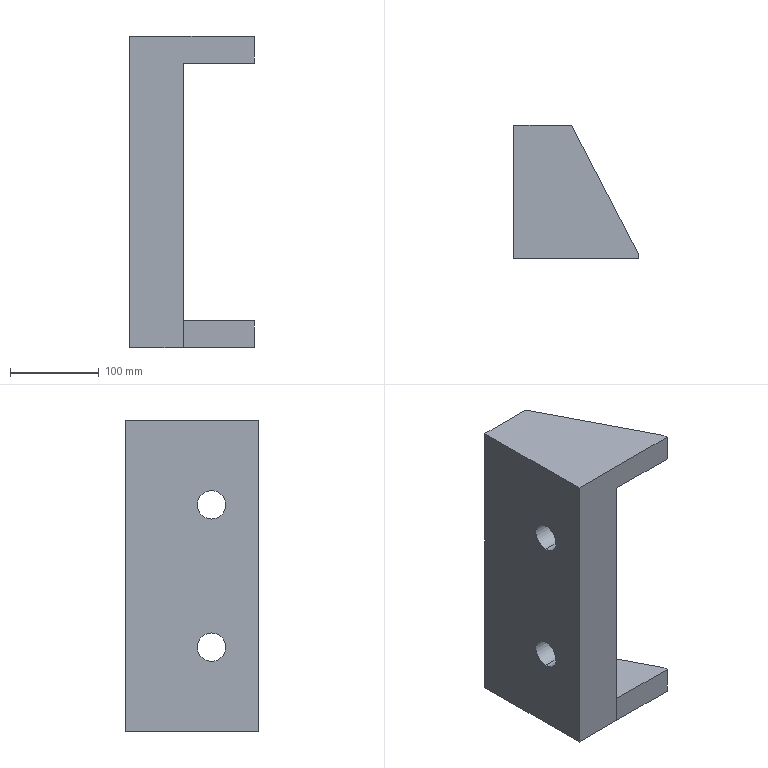Part | STEP file | PN_0005 Linear bearing seat | 2 solids | 20 faces | box 140 x 150 x 350 mm | volume 3447240 mm3 | plane 16 | cylinder 4 | commonest cylinder face diameters 32 x4
STEP:
#1=CARTESIAN_POINT('',(0.,0.,0.));
#2=DIRECTION('',(0.,0.,1.));
#3=DIRECTION('',(1.,0.,0.));
#4=AXIS2_PLACEMENT_3D('',#1,#2,#3);
#5=CARTESIAN_POINT('',(110.,0.,-175.));
#6=VERTEX_POINT('',#5);
#7=CARTESIAN_POINT('',(30.,0.,-175.));
#8=VERTEX_POINT('',#7);
#9=CARTESIAN_POINT('',(30.,0.,-175.));
#10=DIRECTION('',(-1.,0.,0.));
#11=VECTOR('',#10,1.);
#12=LINE('',#9,#11);
#13=CARTESIAN_POINT('',(30.,0.,-145.));
#14=DIRECTION('',(0.,-1.,0.));
#15=DIRECTION('',(1.,0.,0.));
#16=AXIS2_PLACEMENT_3D('',#13,#14,#15);
#17=PLANE('',#16);
#18=CARTESIAN_POINT('',(0.,-30.));
#19=DIRECTION('',(-1.,0.));
#20=VECTOR('',#19,1.);
#21=LINE('',#18,#20);
#22=(GEOMETRIC_REPRESENTATION_CONTEXT(2)PARAMETRIC_REPRESENTATION_CONTEXT()REPRESENTATION_CONTEXT('',''));
#23=DEFINITIONAL_REPRESENTATION('',(#21),#22);
#24=PCURVE('',#17,#23);
#25=CARTESIAN_POINT('',(110.,0.,-175.));
#26=DIRECTION('',(0.,0.,-1.));
#27=DIRECTION('',(-1.,0.,0.));
#28=AXIS2_PLACEMENT_3D('',#25,#26,#27);
#29=PLANE('',#28);
#30=CARTESIAN_POINT('',(80.,0.));
#31=DIRECTION('',(1.,0.));
#32=VECTOR('',#31,1.);
#33=LINE('',#30,#32);
#34=(GEOMETRIC_REPRESENTATION_CONTEXT(2)PARAMETRIC_REPRESENTATION_CONTEXT()REPRESENTATION_CONTEXT('',''));
#35=DEFINITIONAL_REPRESENTATION('',(#33),#34);
#36=PCURVE('',#29,#35);
#37=SURFACE_CURVE('',#12,(#24,#36),.PCURVE_S1.);
#38=EDGE_CURVE('',#6,#8,#37,.T.);
#39=ORIENTED_EDGE('',*,*,#38,.F.);
#40=CARTESIAN_POINT('',(110.,0.,-145.));
#41=VERTEX_POINT('',#40);
#42=CARTESIAN_POINT('',(110.,0.,-145.));
#43=DIRECTION('',(0.,0.,-1.));
#44=VECTOR('',#43,1.);
#45=LINE('',#42,#44);
#46=CARTESIAN_POINT('',(80.,0.));
#47=DIRECTION('',(0.,-1.));
#48=VECTOR('',#47,1.);
#49=LINE('',#46,#48);
#50=(GEOMETRIC_REPRESENTATION_CONTEXT(2)PARAMETRIC_REPRESENTATION_CONTEXT()REPRESENTATION_CONTEXT('',''));
#51=DEFINITIONAL_REPRESENTATION('',(#49),#50);
#52=PCURVE('',#17,#51);
#53=CARTESIAN_POINT('',(110.,5.,-145.));
#54=DIRECTION('',(1.,0.,0.));
#55=DIRECTION('',(0.,0.,-1.));
#56=AXIS2_PLACEMENT_3D('',#53,#54,#55);
#57=PLANE('',#56);
#58=CARTESIAN_POINT('',(0.,-5.));
#59=DIRECTION('',(1.,0.));
#60=VECTOR('',#59,1.);
#61=LINE('',#58,#60);
#62=(GEOMETRIC_REPRESENTATION_CONTEXT(2)PARAMETRIC_REPRESENTATION_CONTEXT()REPRESENTATION_CONTEXT('',''));
#63=DEFINITIONAL_REPRESENTATION('',(#61),#62);
#64=PCURVE('',#57,#63);
#65=SURFACE_CURVE('',#45,(#52,#64),.PCURVE_S1.);
#66=EDGE_CURVE('',#41,#6,#65,.T.);
#67=ORIENTED_EDGE('',*,*,#66,.F.);
#68=CARTESIAN_POINT('',(30.,0.,-145.));
#69=VERTEX_POINT('',#68);
#70=CARTESIAN_POINT('',(30.,0.,-145.));
#71=DIRECTION('',(-1.,0.,0.));
#72=VECTOR('',#71,1.);
#73=LINE('',#70,#72);
#74=CARTESIAN_POINT('',(0.,0.));
#75=DIRECTION('',(-1.,0.));
#76=VECTOR('',#75,1.);
#77=LINE('',#74,#76);
#78=(GEOMETRIC_REPRESENTATION_CONTEXT(2)PARAMETRIC_REPRESENTATION_CONTEXT()REPRESENTATION_CONTEXT('',''));
#79=DEFINITIONAL_REPRESENTATION('',(#77),#78);
#80=PCURVE('',#17,#79);
#81=CARTESIAN_POINT('',(110.,0.,-145.));
#82=DIRECTION('',(0.,0.,-1.));
#83=DIRECTION('',(-1.,0.,0.));
#84=AXIS2_PLACEMENT_3D('',#81,#82,#83);
#85=PLANE('',#84);
#86=CARTESIAN_POINT('',(80.,0.));
#87=DIRECTION('',(1.,0.));
#88=VECTOR('',#87,1.);
#89=LINE('',#86,#88);
#90=(GEOMETRIC_REPRESENTATION_CONTEXT(2)PARAMETRIC_REPRESENTATION_CONTEXT()REPRESENTATION_CONTEXT('',''));
#91=DEFINITIONAL_REPRESENTATION('',(#89),#90);
#92=PCURVE('',#85,#91);
#93=SURFACE_CURVE('',#73,(#80,#92),.PCURVE_S1.);
#94=EDGE_CURVE('',#41,#69,#93,.T.);
#95=ORIENTED_EDGE('',*,*,#94,.T.);
#96=CARTESIAN_POINT('',(30.,0.,-145.));
#97=DIRECTION('',(0.,0.,-1.));
#98=VECTOR('',#97,1.);
#99=LINE('',#96,#98);
#100=CARTESIAN_POINT('',(0.,0.));
#101=DIRECTION('',(0.,-1.));
#102=VECTOR('',#101,1.);
#103=LINE('',#100,#102);
#104=(GEOMETRIC_REPRESENTATION_CONTEXT(2)PARAMETRIC_REPRESENTATION_CONTEXT()REPRESENTATION_CONTEXT('',''));
#105=DEFINITIONAL_REPRESENTATION('',(#103),#104);
#106=PCURVE('',#17,#105);
#107=CARTESIAN_POINT('',(30.,150.,-145.));
#108=DIRECTION('',(-1.,0.,0.));
#109=DIRECTION('',(0.,0.,1.));
#110=AXIS2_PLACEMENT_3D('',#107,#108,#109);
#111=PLANE('',#110);
#112=CARTESIAN_POINT('',(0.,-150.));
#113=DIRECTION('',(-1.,0.));
#114=VECTOR('',#113,1.);
#115=LINE('',#112,#114);
#116=(GEOMETRIC_REPRESENTATION_CONTEXT(2)PARAMETRIC_REPRESENTATION_CONTEXT()REPRESENTATION_CONTEXT('',''));
#117=DEFINITIONAL_REPRESENTATION('',(#115),#116);
#118=PCURVE('',#111,#117);
#119=SURFACE_CURVE('',#99,(#106,#118),.PCURVE_S1.);
#120=EDGE_CURVE('',#69,#8,#119,.T.);
#121=ORIENTED_EDGE('',*,*,#120,.T.);
#122=EDGE_LOOP('',(#39,#67,#95,#121));
#123=FACE_BOUND('',#122,.T.);
#124=ADVANCED_FACE('',(#123),#17,.T.);
#125=CARTESIAN_POINT('',(110.,5.,-175.));
#126=VERTEX_POINT('',#125);
#127=CARTESIAN_POINT('',(110.,5.,-175.));
#128=DIRECTION('',(0.,-1.,0.));
#129=VECTOR('',#128,1.);
#130=LINE('',#127,#129);
#131=CARTESIAN_POINT('',(30.,0.));
#132=DIRECTION('',(0.,-1.));
#133=VECTOR('',#132,1.);
#134=LINE('',#131,#133);
#135=(GEOMETRIC_REPRESENTATION_CONTEXT(2)PARAMETRIC_REPRESENTATION_CONTEXT()REPRESENTATION_CONTEXT('',''));
#136=DEFINITIONAL_REPRESENTATION('',(#134),#135);
#137=PCURVE('',#57,#136);
#138=CARTESIAN_POINT('',(0.,5.));
#139=DIRECTION('',(0.,-1.));
#140=VECTOR('',#139,1.);
#141=LINE('',#138,#140);
#142=(GEOMETRIC_REPRESENTATION_CONTEXT(2)PARAMETRIC_REPRESENTATION_CONTEXT()REPRESENTATION_CONTEXT('',''));
#143=DEFINITIONAL_REPRESENTATION('',(#141),#142);
#144=PCURVE('',#29,#143);
#145=SURFACE_CURVE('',#130,(#137,#144),.PCURVE_S1.);
#146=EDGE_CURVE('',#126,#6,#145,.T.);
#147=ORIENTED_EDGE('',*,*,#146,.F.);
#148=CARTESIAN_POINT('',(110.,5.,-145.));
#149=VERTEX_POINT('',#148);
#150=CARTESIAN_POINT('',(110.,5.,-145.));
#151=DIRECTION('',(0.,0.,-1.));
#152=VECTOR('',#151,1.);
#153=LINE('',#150,#152);
#154=CARTESIAN_POINT('',(0.,0.));
#155=DIRECTION('',(1.,0.));
#156=VECTOR('',#155,1.);
#157=LINE('',#154,#156);
#158=(GEOMETRIC_REPRESENTATION_CONTEXT(2)PARAMETRIC_REPRESENTATION_CONTEXT()REPRESENTATION_CONTEXT('',''));
#159=DEFINITIONAL_REPRESENTATION('',(#157),#158);
#160=PCURVE('',#57,#159);
#161=CARTESIAN_POINT('',(110.,5.,-145.));
#162=DIRECTION('',(0.8882,0.4594,0.));
#163=DIRECTION('',(-0.4594,0.8882,0.));
#164=AXIS2_PLACEMENT_3D('',#161,#162,#163);
#165=PLANE('',#164);
#166=CARTESIAN_POINT('',(0.,0.));
#167=DIRECTION('',(0.,-1.));
#168=VECTOR('',#167,1.);
#169=LINE('',#166,#168);
#170=(GEOMETRIC_REPRESENTATION_CONTEXT(2)PARAMETRIC_REPRESENTATION_CONTEXT()REPRESENTATION_CONTEXT('',''));
#171=DEFINITIONAL_REPRESENTATION('',(#169),#170);
#172=PCURVE('',#165,#171);
#173=SURFACE_CURVE('',#153,(#160,#172),.PCURVE_S1.);
#174=EDGE_CURVE('',#149,#126,#173,.T.);
#175=ORIENTED_EDGE('',*,*,#174,.F.);
#176=CARTESIAN_POINT('',(110.,5.,-145.));
#177=DIRECTION('',(0.,-1.,0.));
#178=VECTOR('',#177,1.);
#179=LINE('',#176,#178);
#180=CARTESIAN_POINT('',(0.,0.));
#181=DIRECTION('',(0.,-1.));
#182=VECTOR('',#181,1.);
#183=LINE('',#180,#182);
#184=(GEOMETRIC_REPRESENTATION_CONTEXT(2)PARAMETRIC_REPRESENTATION_CONTEXT()REPRESENTATION_CONTEXT('',''));
#185=DEFINITIONAL_REPRESENTATION('',(#183),#184);
#186=PCURVE('',#57,#185);
#187=CARTESIAN_POINT('',(0.,5.));
#188=DIRECTION('',(0.,-1.));
#189=VECTOR('',#188,1.);
#190=LINE('',#187,#189);
#191=(GEOMETRIC_REPRESENTATION_CONTEXT(2)PARAMETRIC_REPRESENTATION_CONTEXT()REPRESENTATION_CONTEXT('',''));
#192=DEFINITIONAL_REPRESENTATION('',(#190),#191);
#193=PCURVE('',#85,#192);
#194=SURFACE_CURVE('',#179,(#186,#193),.PCURVE_S1.);
#195=EDGE_CURVE('',#149,#41,#194,.T.);
#196=ORIENTED_EDGE('',*,*,#195,.T.);
#197=ORIENTED_EDGE('',*,*,#66,.T.);
#198=EDGE_LOOP('',(#147,#175,#196,#197));
#199=FACE_BOUND('',#198,.T.);
#200=ADVANCED_FACE('',(#199),#57,.T.);
#201=CARTESIAN_POINT('',(35.,150.,-175.));
#202=VERTEX_POINT('',#201);
#203=CARTESIAN_POINT('',(110.,5.,-175.));
#204=DIRECTION('',(0.4594,-0.8882,0.));
#205=VECTOR('',#204,1.);
#206=LINE('',#203,#205);
#207=CARTESIAN_POINT('',(0.,-30.));
#208=DIRECTION('',(-1.,0.));
#209=VECTOR('',#208,1.);
#210=LINE('',#207,#209);
#211=(GEOMETRIC_REPRESENTATION_CONTEXT(2)PARAMETRIC_REPRESENTATION_CONTEXT()REPRESENTATION_CONTEXT('',''));
#212=DEFINITIONAL_REPRESENTATION('',(#210),#211);
#213=PCURVE('',#165,#212);
#214=CARTESIAN_POINT('',(0.,5.));
#215=DIRECTION('',(-0.4594,-0.8882));
#216=VECTOR('',#215,1.);
#217=LINE('',#214,#216);
#218=(GEOMETRIC_REPRESENTATION_CONTEXT(2)PARAMETRIC_REPRESENTATION_CONTEXT()REPRESENTATION_CONTEXT('',''));
#219=DEFINITIONAL_REPRESENTATION('',(#217),#218);
#220=PCURVE('',#29,#219);
#221=SURFACE_CURVE('',#206,(#213,#220),.PCURVE_S1.);
#222=EDGE_CURVE('',#202,#126,#221,.T.);
#223=ORIENTED_EDGE('',*,*,#222,.F.);
#224=CARTESIAN_POINT('',(35.,150.,-145.));
#225=VERTEX_POINT('',#224);
#226=CARTESIAN_POINT('',(35.,150.,-145.));
#227=DIRECTION('',(0.,0.,-1.));
#228=VECTOR('',#227,1.);
#229=LINE('',#226,#228);
#230=CARTESIAN_POINT('',(163.248,0.));
#231=DIRECTION('',(0.,-1.));
#232=VECTOR('',#231,1.);
#233=LINE('',#230,#232);
#234=(GEOMETRIC_REPRESENTATION_CONTEXT(2)PARAMETRIC_REPRESENTATION_CONTEXT()REPRESENTATION_CONTEXT('',''));
#235=DEFINITIONAL_REPRESENTATION('',(#233),#234);
#236=PCURVE('',#165,#235);
#237=CARTESIAN_POINT('',(35.,150.,-145.));
#238=DIRECTION('',(0.,1.,0.));
#239=DIRECTION('',(-1.,0.,0.));
#240=AXIS2_PLACEMENT_3D('',#237,#238,#239);
#241=PLANE('',#240);
#242=CARTESIAN_POINT('',(0.,0.));
#243=DIRECTION('',(0.,-1.));
#244=VECTOR('',#243,1.);
#245=LINE('',#242,#244);
#246=(GEOMETRIC_REPRESENTATION_CONTEXT(2)PARAMETRIC_REPRESENTATION_CONTEXT()REPRESENTATION_CONTEXT('',''));
#247=DEFINITIONAL_REPRESENTATION('',(#245),#246);
#248=PCURVE('',#241,#247);
#249=SURFACE_CURVE('',#229,(#236,#248),.PCURVE_S1.);
#250=EDGE_CURVE('',#225,#202,#249,.T.);
#251=ORIENTED_EDGE('',*,*,#250,.F.);
#252=CARTESIAN_POINT('',(110.,5.,-145.));
#253=DIRECTION('',(0.4594,-0.8882,0.));
#254=VECTOR('',#253,1.);
#255=LINE('',#252,#254);
#256=CARTESIAN_POINT('',(0.,0.));
#257=DIRECTION('',(-1.,0.));
#258=VECTOR('',#257,1.);
#259=LINE('',#256,#258);
#260=(GEOMETRIC_REPRESENTATION_CONTEXT(2)PARAMETRIC_REPRESENTATION_CONTEXT()REPRESENTATION_CONTEXT('',''));
#261=DEFINITIONAL_REPRESENTATION('',(#259),#260);
#262=PCURVE('',#165,#261);
#263=CARTESIAN_POINT('',(0.,5.));
#264=DIRECTION('',(-0.4594,-0.8882));
#265=VECTOR('',#264,1.);
#266=LINE('',#263,#265);
#267=(GEOMETRIC_REPRESENTATION_CONTEXT(2)PARAMETRIC_REPRESENTATION_CONTEXT()REPRESENTATION_CONTEXT('',''));
#268=DEFINITIONAL_REPRESENTATION('',(#266),#267);
#269=PCURVE('',#85,#268);
#270=SURFACE_CURVE('',#255,(#262,#269),.PCURVE_S1.);
#271=EDGE_CURVE('',#225,#149,#270,.T.);
#272=ORIENTED_EDGE('',*,*,#271,.T.);
#273=ORIENTED_EDGE('',*,*,#174,.T.);
#274=EDGE_LOOP('',(#223,#251,#272,#273));
#275=FACE_BOUND('',#274,.T.);
#276=ADVANCED_FACE('',(#275),#165,.T.);
#277=CARTESIAN_POINT('',(30.,150.,-175.));
#278=VERTEX_POINT('',#277);
#279=CARTESIAN_POINT('',(35.,150.,-175.));
#280=DIRECTION('',(1.,0.,0.));
#281=VECTOR('',#280,1.);
#282=LINE('',#279,#281);
#283=CARTESIAN_POINT('',(0.,-30.));
#284=DIRECTION('',(-1.,0.));
#285=VECTOR('',#284,1.);
#286=LINE('',#283,#285);
#287=(GEOMETRIC_REPRESENTATION_CONTEXT(2)PARAMETRIC_REPRESENTATION_CONTEXT()REPRESENTATION_CONTEXT('',''));
#288=DEFINITIONAL_REPRESENTATION('',(#286),#287);
#289=PCURVE('',#241,#288);
#290=CARTESIAN_POINT('',(75.,150.));
#291=DIRECTION('',(-1.,0.));
#292=VECTOR('',#291,1.);
#293=LINE('',#290,#292);
#294=(GEOMETRIC_REPRESENTATION_CONTEXT(2)PARAMETRIC_REPRESENTATION_CONTEXT()REPRESENTATION_CONTEXT('',''));
#295=DEFINITIONAL_REPRESENTATION('',(#293),#294);
#296=PCURVE('',#29,#295);
#297=SURFACE_CURVE('',#282,(#289,#296),.PCURVE_S1.);
#298=EDGE_CURVE('',#278,#202,#297,.T.);
#299=ORIENTED_EDGE('',*,*,#298,.F.);
#300=CARTESIAN_POINT('',(30.,150.,-145.));
#301=VERTEX_POINT('',#300);
#302=CARTESIAN_POINT('',(30.,150.,-145.));
#303=DIRECTION('',(0.,0.,-1.));
#304=VECTOR('',#303,1.);
#305=LINE('',#302,#304);
#306=CARTESIAN_POINT('',(5.,0.));
#307=DIRECTION('',(0.,-1.));
#308=VECTOR('',#307,1.);
#309=LINE('',#306,#308);
#310=(GEOMETRIC_REPRESENTATION_CONTEXT(2)PARAMETRIC_REPRESENTATION_CONTEXT()REPRESENTATION_CONTEXT('',''));
#311=DEFINITIONAL_REPRESENTATION('',(#309),#310);
#312=PCURVE('',#241,#311);
#313=CARTESIAN_POINT('',(0.,0.));
#314=DIRECTION('',(-1.,0.));
#315=VECTOR('',#314,1.);
#316=LINE('',#313,#315);
#317=(GEOMETRIC_REPRESENTATION_CONTEXT(2)PARAMETRIC_REPRESENTATION_CONTEXT()REPRESENTATION_CONTEXT('',''));
#318=DEFINITIONAL_REPRESENTATION('',(#316),#317);
#319=PCURVE('',#111,#318);
#320=SURFACE_CURVE('',#305,(#312,#319),.PCURVE_S1.);
#321=EDGE_CURVE('',#301,#278,#320,.T.);
#322=ORIENTED_EDGE('',*,*,#321,.F.);
#323=CARTESIAN_POINT('',(35.,150.,-145.));
#324=DIRECTION('',(1.,0.,0.));
#325=VECTOR('',#324,1.);
#326=LINE('',#323,#325);
#327=CARTESIAN_POINT('',(0.,0.));
#328=DIRECTION('',(-1.,0.));
#329=VECTOR('',#328,1.);
#330=LINE('',#327,#329);
#331=(GEOMETRIC_REPRESENTATION_CONTEXT(2)PARAMETRIC_REPRESENTATION_CONTEXT()REPRESENTATION_CONTEXT('',''));
#332=DEFINITIONAL_REPRESENTATION('',(#330),#331);
#333=PCURVE('',#241,#332);
#334=CARTESIAN_POINT('',(75.,150.));
#335=DIRECTION('',(-1.,0.));
#336=VECTOR('',#335,1.);
#337=LINE('',#334,#336);
#338=(GEOMETRIC_REPRESENTATION_CONTEXT(2)PARAMETRIC_REPRESENTATION_CONTEXT()REPRESENTATION_CONTEXT('',''));
#339=DEFINITIONAL_REPRESENTATION('',(#337),#338);
#340=PCURVE('',#85,#339);
#341=SURFACE_CURVE('',#326,(#333,#340),.PCURVE_S1.);
#342=EDGE_CURVE('',#301,#225,#341,.T.);
#343=ORIENTED_EDGE('',*,*,#342,.T.);
#344=ORIENTED_EDGE('',*,*,#250,.T.);
#345=EDGE_LOOP('',(#299,#322,#343,#344));
#346=FACE_BOUND('',#345,.T.);
#347=ADVANCED_FACE('',(#346),#241,.T.);
#348=CARTESIAN_POINT('',(30.,150.,-175.));
#349=DIRECTION('',(0.,1.,0.));
#350=VECTOR('',#349,1.);
#351=LINE('',#348,#350);
#352=CARTESIAN_POINT('',(-30.,0.));
#353=DIRECTION('',(0.,1.));
#354=VECTOR('',#353,1.);
#355=LINE('',#352,#354);
#356=(GEOMETRIC_REPRESENTATION_CONTEXT(2)PARAMETRIC_REPRESENTATION_CONTEXT()REPRESENTATION_CONTEXT('',''));
#357=DEFINITIONAL_REPRESENTATION('',(#355),#356);
#358=PCURVE('',#111,#357);
#359=CARTESIAN_POINT('',(80.,150.));
#360=DIRECTION('',(0.,1.));
#361=VECTOR('',#360,1.);
#362=LINE('',#359,#361);
#363=(GEOMETRIC_REPRESENTATION_CONTEXT(2)PARAMETRIC_REPRESENTATION_CONTEXT()REPRESENTATION_CONTEXT('',''));
#364=DEFINITIONAL_REPRESENTATION('',(#362),#363);
#365=PCURVE('',#29,#364);
#366=SURFACE_CURVE('',#351,(#358,#365),.PCURVE_S1.);
#367=EDGE_CURVE('',#8,#278,#366,.T.);
#368=ORIENTED_EDGE('',*,*,#367,.F.);
#369=ORIENTED_EDGE('',*,*,#120,.F.);
#370=CARTESIAN_POINT('',(30.,150.,-145.));
#371=DIRECTION('',(0.,1.,0.));
#372=VECTOR('',#371,1.);
#373=LINE('',#370,#372);
#374=CARTESIAN_POINT('',(0.,0.));
#375=DIRECTION('',(0.,1.));
#376=VECTOR('',#375,1.);
#377=LINE('',#374,#376);
#378=(GEOMETRIC_REPRESENTATION_CONTEXT(2)PARAMETRIC_REPRESENTATION_CONTEXT()REPRESENTATION_CONTEXT('',''));
#379=DEFINITIONAL_REPRESENTATION('',(#377),#378);
#380=PCURVE('',#111,#379);
#381=CARTESIAN_POINT('',(80.,150.));
#382=DIRECTION('',(0.,1.));
#383=VECTOR('',#382,1.);
#384=LINE('',#381,#383);
#385=(GEOMETRIC_REPRESENTATION_CONTEXT(2)PARAMETRIC_REPRESENTATION_CONTEXT()REPRESENTATION_CONTEXT('',''));
#386=DEFINITIONAL_REPRESENTATION('',(#384),#385);
#387=PCURVE('',#85,#386);
#388=SURFACE_CURVE('',#373,(#380,#387),.PCURVE_S1.);
#389=EDGE_CURVE('',#69,#301,#388,.T.);
#390=ORIENTED_EDGE('',*,*,#389,.T.);
#391=ORIENTED_EDGE('',*,*,#321,.T.);
#392=EDGE_LOOP('',(#368,#369,#390,#391));
#393=FACE_BOUND('',#392,.T.);
#394=ADVANCED_FACE('',(#393),#111,.T.);
#395=ORIENTED_EDGE('',*,*,#94,.F.);
#396=ORIENTED_EDGE('',*,*,#195,.F.);
#397=ORIENTED_EDGE('',*,*,#271,.F.);
#398=ORIENTED_EDGE('',*,*,#342,.F.);
#399=ORIENTED_EDGE('',*,*,#389,.F.);
#400=EDGE_LOOP('',(#395,#396,#397,#398,#399));
#401=FACE_BOUND('',#400,.T.);
#402=ADVANCED_FACE('',(#401),#85,.F.);
#403=ORIENTED_EDGE('',*,*,#38,.T.);
#404=ORIENTED_EDGE('',*,*,#367,.T.);
#405=ORIENTED_EDGE('',*,*,#298,.T.);
#406=ORIENTED_EDGE('',*,*,#222,.T.);
#407=ORIENTED_EDGE('',*,*,#146,.T.);
#408=EDGE_LOOP('',(#403,#404,#405,#406,#407));
#409=FACE_BOUND('',#408,.T.);
#410=ADVANCED_FACE('',(#409),#29,.T.);
#411=CLOSED_SHELL('',(#124,#200,#276,#347,#394,#402,#410));
#412=MANIFOLD_SOLID_BREP('',#411);
#413=CARTESIAN_POINT('',(30.,53.,96.));
#414=VERTEX_POINT('',#413);
#415=CARTESIAN_POINT('',(-30.,53.,96.));
#416=VERTEX_POINT('',#415);
#417=CARTESIAN_POINT('',(30.,53.,96.));
#418=DIRECTION('',(-1.,0.,0.));
#419=VECTOR('',#418,1.);
#420=LINE('',#417,#419);
#421=CARTESIAN_POINT('',(30.,53.,80.));
#422=DIRECTION('',(-1.,0.,0.));
#423=DIRECTION('',(0.,0.,1.));
#424=AXIS2_PLACEMENT_3D('',#421,#422,#423);
#425=CYLINDRICAL_SURFACE('',#424,16.);
#426=CARTESIAN_POINT('',(6.283,0.));
#427=DIRECTION('',(0.,1.));
#428=VECTOR('',#427,1.);
#429=LINE('',#426,#428);
#430=(GEOMETRIC_REPRESENTATION_CONTEXT(2)PARAMETRIC_REPRESENTATION_CONTEXT()REPRESENTATION_CONTEXT('',''));
#431=DEFINITIONAL_REPRESENTATION('',(#429),#430);
#432=PCURVE('',#425,#431);
#433=CARTESIAN_POINT('',(30.,53.,80.));
#434=DIRECTION('',(-1.,0.,0.));
#435=DIRECTION('',(0.,0.,1.));
#436=AXIS2_PLACEMENT_3D('',#433,#434,#435);
#437=CYLINDRICAL_SURFACE('',#436,16.);
#438=CARTESIAN_POINT('',(0.,0.));
#439=DIRECTION('',(0.,1.));
#440=VECTOR('',#439,1.);
#441=LINE('',#438,#440);
#442=(GEOMETRIC_REPRESENTATION_CONTEXT(2)PARAMETRIC_REPRESENTATION_CONTEXT()REPRESENTATION_CONTEXT('',''));
#443=DEFINITIONAL_REPRESENTATION('',(#441),#442);
#444=PCURVE('',#437,#443);
#445=SURFACE_CURVE('',#420,(#432,#444),.PCURVE_S1.);
#446=EDGE_CURVE('',#414,#416,#445,.T.);
#447=ORIENTED_EDGE('',*,*,#446,.T.);
#448=CARTESIAN_POINT('',(-30.,53.,64.));
#449=VERTEX_POINT('',#448);
#450=CARTESIAN_POINT('',(-30.,53.,80.));
#451=DIRECTION('',(-1.,0.,0.));
#452=DIRECTION('',(0.,0.,1.));
#453=AXIS2_PLACEMENT_3D('',#450,#451,#452);
#454=CIRCLE('',#453,16.);
#455=CARTESIAN_POINT('',(0.,60.));
#456=DIRECTION('',(1.,0.));
#457=VECTOR('',#456,1.);
#458=LINE('',#455,#457);
#459=(GEOMETRIC_REPRESENTATION_CONTEXT(2)PARAMETRIC_REPRESENTATION_CONTEXT()REPRESENTATION_CONTEXT('',''));
#460=DEFINITIONAL_REPRESENTATION('',(#458),#459);
#461=PCURVE('',#425,#460);
#462=CARTESIAN_POINT('',(-30.,150.,-175.));
#463=DIRECTION('',(1.,0.,0.));
#464=DIRECTION('',(0.,0.,-1.));
#465=AXIS2_PLACEMENT_3D('',#462,#463,#464);
#466=PLANE('',#465);
#467=CARTESIAN_POINT('',(-271.,-97.));
#468=CARTESIAN_POINT('',(-271.,-69.287));
#469=CARTESIAN_POINT('',(-247.,-83.144));
#470=CARTESIAN_POINT('',(-223.,-97.));
#471=CARTESIAN_POINT('',(-247.,-110.856));
#472=CARTESIAN_POINT('',(-271.,-124.713));
#473=CARTESIAN_POINT('',(-271.,-97.));
#474=(BOUNDED_CURVE()B_SPLINE_CURVE(2,(#467,#468,#469,#470,#471,#472,#473),.UNSPECIFIED.,.T.,.F.)B_SPLINE_CURVE_WITH_KNOTS((1,2,2,2,2,1),(-2.094,0.,2.094,4.189,6.283,8.378),.UNSPECIFIED.)CURVE()GEOMETRIC_REPRESENTATION_ITEM()RATIONAL_B_SPLINE_CURVE((1.,0.5,1.,0.5,1.,0.5,1.))REPRESENTATION_ITEM(''));
#475=(GEOMETRIC_REPRESENTATION_CONTEXT(2)PARAMETRIC_REPRESENTATION_CONTEXT()REPRESENTATION_CONTEXT('',''));
#476=DEFINITIONAL_REPRESENTATION('',(#474),#475);
#477=PCURVE('',#466,#476);
#478=SURFACE_CURVE('',#454,(#461,#477),.PCURVE_S1.);
#479=EDGE_CURVE('',#449,#416,#478,.T.);
#480=ORIENTED_EDGE('',*,*,#479,.F.);
#481=CARTESIAN_POINT('',(30.,53.,64.));
#482=VERTEX_POINT('',#481);
#483=CARTESIAN_POINT('',(30.,53.,64.));
#484=DIRECTION('',(-1.,0.,0.));
#485=VECTOR('',#484,1.);
#486=LINE('',#483,#485);
#487=CARTESIAN_POINT('',(3.142,0.));
#488=DIRECTION('',(0.,1.));
#489=VECTOR('',#488,1.);
#490=LINE('',#487,#489);
#491=(GEOMETRIC_REPRESENTATION_CONTEXT(2)PARAMETRIC_REPRESENTATION_CONTEXT()REPRESENTATION_CONTEXT('',''));
#492=DEFINITIONAL_REPRESENTATION('',(#490),#491);
#493=PCURVE('',#425,#492);
#494=CARTESIAN_POINT('',(3.142,0.));
#495=DIRECTION('',(0.,1.));
#496=VECTOR('',#495,1.);
#497=LINE('',#494,#496);
#498=(GEOMETRIC_REPRESENTATION_CONTEXT(2)PARAMETRIC_REPRESENTATION_CONTEXT()REPRESENTATION_CONTEXT('',''));
#499=DEFINITIONAL_REPRESENTATION('',(#497),#498);
#500=PCURVE('',#437,#499);
#501=SURFACE_CURVE('',#486,(#493,#500),.PCURVE_S1.);
#502=EDGE_CURVE('',#482,#449,#501,.T.);
#503=ORIENTED_EDGE('',*,*,#502,.F.);
#504=CARTESIAN_POINT('',(30.,53.,80.));
#505=DIRECTION('',(-1.,0.,0.));
#506=DIRECTION('',(0.,0.,1.));
#507=AXIS2_PLACEMENT_3D('',#504,#505,#506);
#508=CIRCLE('',#507,16.);
#509=CARTESIAN_POINT('',(0.,0.));
#510=DIRECTION('',(1.,0.));
#511=VECTOR('',#510,1.);
#512=LINE('',#509,#511);
#513=(GEOMETRIC_REPRESENTATION_CONTEXT(2)PARAMETRIC_REPRESENTATION_CONTEXT()REPRESENTATION_CONTEXT('',''));
#514=DEFINITIONAL_REPRESENTATION('',(#512),#513);
#515=PCURVE('',#425,#514);
#516=CARTESIAN_POINT('',(30.,150.,-175.));
#517=DIRECTION('',(-1.,0.,0.));
#518=DIRECTION('',(0.,0.,1.));
#519=AXIS2_PLACEMENT_3D('',#516,#517,#518);
#520=PLANE('',#519);
#521=CARTESIAN_POINT('',(255.,-97.));
#522=DIRECTION('',(1.,0.));
#523=AXIS2_PLACEMENT_2D('',#521,#522);
#524=CIRCLE('',#523,16.);
#525=(GEOMETRIC_REPRESENTATION_CONTEXT(2)PARAMETRIC_REPRESENTATION_CONTEXT()REPRESENTATION_CONTEXT('',''));
#526=DEFINITIONAL_REPRESENTATION('',(#524),#525);
#527=PCURVE('',#520,#526);
#528=SURFACE_CURVE('',#508,(#515,#527),.PCURVE_S1.);
#529=EDGE_CURVE('',#482,#414,#528,.T.);
#530=ORIENTED_EDGE('',*,*,#529,.T.);
#531=EDGE_LOOP('',(#447,#480,#503,#530));
#532=FACE_BOUND('',#531,.F.);
#533=ADVANCED_FACE('',(#532),#425,.F.);
#534=CARTESIAN_POINT('',(30.,53.,-64.));
#535=VERTEX_POINT('',#534);
#536=CARTESIAN_POINT('',(-30.,53.,-64.));
#537=VERTEX_POINT('',#536);
#538=CARTESIAN_POINT('',(30.,53.,-64.));
#539=DIRECTION('',(-1.,0.,0.));
#540=VECTOR('',#539,1.);
#541=LINE('',#538,#540);
#542=CARTESIAN_POINT('',(30.,53.,-80.));
#543=DIRECTION('',(-1.,0.,0.));
#544=DIRECTION('',(0.,0.,1.));
#545=AXIS2_PLACEMENT_3D('',#542,#543,#544);
#546=CYLINDRICAL_SURFACE('',#545,16.);
#547=CARTESIAN_POINT('',(6.283,0.));
#548=DIRECTION('',(0.,1.));
#549=VECTOR('',#548,1.);
#550=LINE('',#547,#549);
#551=(GEOMETRIC_REPRESENTATION_CONTEXT(2)PARAMETRIC_REPRESENTATION_CONTEXT()REPRESENTATION_CONTEXT('',''));
#552=DEFINITIONAL_REPRESENTATION('',(#550),#551);
#553=PCURVE('',#546,#552);
#554=CARTESIAN_POINT('',(30.,53.,-80.));
#555=DIRECTION('',(-1.,0.,0.));
#556=DIRECTION('',(0.,0.,1.));
#557=AXIS2_PLACEMENT_3D('',#554,#555,#556);
#558=CYLINDRICAL_SURFACE('',#557,16.);
#559=CARTESIAN_POINT('',(0.,0.));
#560=DIRECTION('',(0.,1.));
#561=VECTOR('',#560,1.);
#562=LINE('',#559,#561);
#563=(GEOMETRIC_REPRESENTATION_CONTEXT(2)PARAMETRIC_REPRESENTATION_CONTEXT()REPRESENTATION_CONTEXT('',''));
#564=DEFINITIONAL_REPRESENTATION('',(#562),#563);
#565=PCURVE('',#558,#564);
#566=SURFACE_CURVE('',#541,(#553,#565),.PCURVE_S1.);
#567=EDGE_CURVE('',#535,#537,#566,.T.);
#568=ORIENTED_EDGE('',*,*,#567,.T.);
#569=CARTESIAN_POINT('',(-30.,53.,-96.));
#570=VERTEX_POINT('',#569);
#571=CARTESIAN_POINT('',(-30.,53.,-80.));
#572=DIRECTION('',(-1.,0.,0.));
#573=DIRECTION('',(0.,0.,1.));
#574=AXIS2_PLACEMENT_3D('',#571,#572,#573);
#575=CIRCLE('',#574,16.);
#576=CARTESIAN_POINT('',(0.,60.));
#577=DIRECTION('',(1.,0.));
#578=VECTOR('',#577,1.);
#579=LINE('',#576,#578);
#580=(GEOMETRIC_REPRESENTATION_CONTEXT(2)PARAMETRIC_REPRESENTATION_CONTEXT()REPRESENTATION_CONTEXT('',''));
#581=DEFINITIONAL_REPRESENTATION('',(#579),#580);
#582=PCURVE('',#546,#581);
#583=CARTESIAN_POINT('',(-111.,-97.));
#584=CARTESIAN_POINT('',(-111.,-69.287));
#585=CARTESIAN_POINT('',(-87.,-83.144));
#586=CARTESIAN_POINT('',(-63.,-97.));
#587=CARTESIAN_POINT('',(-87.,-110.856));
#588=CARTESIAN_POINT('',(-111.,-124.713));
#589=CARTESIAN_POINT('',(-111.,-97.));
#590=(BOUNDED_CURVE()B_SPLINE_CURVE(2,(#583,#584,#585,#586,#587,#588,#589),.UNSPECIFIED.,.T.,.F.)B_SPLINE_CURVE_WITH_KNOTS((1,2,2,2,2,1),(-2.094,0.,2.094,4.189,6.283,8.378),.UNSPECIFIED.)CURVE()GEOMETRIC_REPRESENTATION_ITEM()RATIONAL_B_SPLINE_CURVE((1.,0.5,1.,0.5,1.,0.5,1.))REPRESENTATION_ITEM(''));
#591=(GEOMETRIC_REPRESENTATION_CONTEXT(2)PARAMETRIC_REPRESENTATION_CONTEXT()REPRESENTATION_CONTEXT('',''));
#592=DEFINITIONAL_REPRESENTATION('',(#590),#591);
#593=PCURVE('',#466,#592);
#594=SURFACE_CURVE('',#575,(#582,#593),.PCURVE_S1.);
#595=EDGE_CURVE('',#570,#537,#594,.T.);
#596=ORIENTED_EDGE('',*,*,#595,.F.);
#597=CARTESIAN_POINT('',(30.,53.,-96.));
#598=VERTEX_POINT('',#597);
#599=CARTESIAN_POINT('',(30.,53.,-96.));
#600=DIRECTION('',(-1.,0.,0.));
#601=VECTOR('',#600,1.);
#602=LINE('',#599,#601);
#603=CARTESIAN_POINT('',(3.142,0.));
#604=DIRECTION('',(0.,1.));
#605=VECTOR('',#604,1.);
#606=LINE('',#603,#605);
#607=(GEOMETRIC_REPRESENTATION_CONTEXT(2)PARAMETRIC_REPRESENTATION_CONTEXT()REPRESENTATION_CONTEXT('',''));
#608=DEFINITIONAL_REPRESENTATION('',(#606),#607);
#609=PCURVE('',#546,#608);
#610=CARTESIAN_POINT('',(3.142,0.));
#611=DIRECTION('',(0.,1.));
#612=VECTOR('',#611,1.);
#613=LINE('',#610,#612);
#614=(GEOMETRIC_REPRESENTATION_CONTEXT(2)PARAMETRIC_REPRESENTATION_CONTEXT()REPRESENTATION_CONTEXT('',''));
#615=DEFINITIONAL_REPRESENTATION('',(#613),#614);
#616=PCURVE('',#558,#615);
#617=SURFACE_CURVE('',#602,(#609,#616),.PCURVE_S1.);
#618=EDGE_CURVE('',#598,#570,#617,.T.);
#619=ORIENTED_EDGE('',*,*,#618,.F.);
#620=CARTESIAN_POINT('',(30.,53.,-80.));
#621=DIRECTION('',(-1.,0.,0.));
#622=DIRECTION('',(0.,0.,1.));
#623=AXIS2_PLACEMENT_3D('',#620,#621,#622);
#624=CIRCLE('',#623,16.);
#625=CARTESIAN_POINT('',(0.,0.));
#626=DIRECTION('',(1.,0.));
#627=VECTOR('',#626,1.);
#628=LINE('',#625,#627);
#629=(GEOMETRIC_REPRESENTATION_CONTEXT(2)PARAMETRIC_REPRESENTATION_CONTEXT()REPRESENTATION_CONTEXT('',''));
#630=DEFINITIONAL_REPRESENTATION('',(#628),#629);
#631=PCURVE('',#546,#630);
#632=CARTESIAN_POINT('',(95.,-97.));
#633=DIRECTION('',(1.,0.));
#634=AXIS2_PLACEMENT_2D('',#632,#633);
#635=CIRCLE('',#634,16.);
#636=(GEOMETRIC_REPRESENTATION_CONTEXT(2)PARAMETRIC_REPRESENTATION_CONTEXT()REPRESENTATION_CONTEXT('',''));
#637=DEFINITIONAL_REPRESENTATION('',(#635),#636);
#638=PCURVE('',#520,#637);
#639=SURFACE_CURVE('',#624,(#631,#638),.PCURVE_S1.);
#640=EDGE_CURVE('',#598,#535,#639,.T.);
#641=ORIENTED_EDGE('',*,*,#640,.T.);
#642=EDGE_LOOP('',(#568,#596,#619,#641));
#643=FACE_BOUND('',#642,.F.);
#644=ADVANCED_FACE('',(#643),#546,.F.);
#645=CARTESIAN_POINT('',(30.,53.,-80.));
#646=DIRECTION('',(-1.,0.,0.));
#647=DIRECTION('',(0.,0.,1.));
#648=AXIS2_PLACEMENT_3D('',#645,#646,#647);
#649=CIRCLE('',#648,16.);
#650=CARTESIAN_POINT('',(95.,-97.));
#651=DIRECTION('',(1.,0.));
#652=AXIS2_PLACEMENT_2D('',#650,#651);
#653=CIRCLE('',#652,16.);
#654=(GEOMETRIC_REPRESENTATION_CONTEXT(2)PARAMETRIC_REPRESENTATION_CONTEXT()REPRESENTATION_CONTEXT('',''));
#655=DEFINITIONAL_REPRESENTATION('',(#653),#654);
#656=PCURVE('',#520,#655);
#657=CARTESIAN_POINT('',(0.,0.));
#658=DIRECTION('',(1.,0.));
#659=VECTOR('',#658,1.);
#660=LINE('',#657,#659);
#661=(GEOMETRIC_REPRESENTATION_CONTEXT(2)PARAMETRIC_REPRESENTATION_CONTEXT()REPRESENTATION_CONTEXT('',''));
#662=DEFINITIONAL_REPRESENTATION('',(#660),#661);
#663=PCURVE('',#558,#662);
#664=SURFACE_CURVE('',#649,(#656,#663),.PCURVE_S1.);
#665=EDGE_CURVE('',#535,#598,#664,.T.);
#666=ORIENTED_EDGE('',*,*,#665,.T.);
#667=ORIENTED_EDGE('',*,*,#640,.T.);
#668=EDGE_LOOP('',(#666,#667));
#669=FACE_BOUND('',#668,.T.);
#670=CARTESIAN_POINT('',(30.,53.,80.));
#671=DIRECTION('',(-1.,0.,0.));
#672=DIRECTION('',(0.,0.,1.));
#673=AXIS2_PLACEMENT_3D('',#670,#671,#672);
#674=CIRCLE('',#673,16.);
#675=CARTESIAN_POINT('',(255.,-97.));
#676=DIRECTION('',(1.,0.));
#677=AXIS2_PLACEMENT_2D('',#675,#676);
#678=CIRCLE('',#677,16.);
#679=(GEOMETRIC_REPRESENTATION_CONTEXT(2)PARAMETRIC_REPRESENTATION_CONTEXT()REPRESENTATION_CONTEXT('',''));
#680=DEFINITIONAL_REPRESENTATION('',(#678),#679);
#681=PCURVE('',#520,#680);
#682=CARTESIAN_POINT('',(0.,0.));
#683=DIRECTION('',(1.,0.));
#684=VECTOR('',#683,1.);
#685=LINE('',#682,#684);
#686=(GEOMETRIC_REPRESENTATION_CONTEXT(2)PARAMETRIC_REPRESENTATION_CONTEXT()REPRESENTATION_CONTEXT('',''));
#687=DEFINITIONAL_REPRESENTATION('',(#685),#686);
#688=PCURVE('',#437,#687);
#689=SURFACE_CURVE('',#674,(#681,#688),.PCURVE_S1.);
#690=EDGE_CURVE('',#414,#482,#689,.T.);
#691=ORIENTED_EDGE('',*,*,#690,.T.);
#692=ORIENTED_EDGE('',*,*,#529,.T.);
#693=EDGE_LOOP('',(#691,#692));
#694=FACE_BOUND('',#693,.T.);
#695=CARTESIAN_POINT('',(30.,0.,145.));
#696=VERTEX_POINT('',#695);
#697=CARTESIAN_POINT('',(30.,150.,145.));
#698=VERTEX_POINT('',#697);
#699=CARTESIAN_POINT('',(30.,150.,145.));
#700=DIRECTION('',(0.,1.,0.));
#701=VECTOR('',#700,1.);
#702=LINE('',#699,#701);
#703=CARTESIAN_POINT('',(320.,0.));
#704=DIRECTION('',(0.,1.));
#705=VECTOR('',#704,1.);
#706=LINE('',#703,#705);
#707=(GEOMETRIC_REPRESENTATION_CONTEXT(2)PARAMETRIC_REPRESENTATION_CONTEXT()REPRESENTATION_CONTEXT('',''));
#708=DEFINITIONAL_REPRESENTATION('',(#706),#707);
#709=PCURVE('',#520,#708);
#710=CARTESIAN_POINT('',(110.,0.,145.));
#711=DIRECTION('',(0.,0.,-1.));
#712=DIRECTION('',(-1.,0.,0.));
#713=AXIS2_PLACEMENT_3D('',#710,#711,#712);
#714=PLANE('',#713);
#715=CARTESIAN_POINT('',(80.,150.));
#716=DIRECTION('',(0.,1.));
#717=VECTOR('',#716,1.);
#718=LINE('',#715,#717);
#719=(GEOMETRIC_REPRESENTATION_CONTEXT(2)PARAMETRIC_REPRESENTATION_CONTEXT()REPRESENTATION_CONTEXT('',''));
#720=DEFINITIONAL_REPRESENTATION('',(#718),#719);
#721=PCURVE('',#714,#720);
#722=SURFACE_CURVE('',#702,(#709,#721),.PCURVE_S1.);
#723=EDGE_CURVE('',#696,#698,#722,.T.);
#724=ORIENTED_EDGE('',*,*,#723,.F.);
#725=CARTESIAN_POINT('',(30.,0.,-175.));
#726=VERTEX_POINT('',#725);
#727=CARTESIAN_POINT('',(30.,0.,-175.));
#728=DIRECTION('',(0.,0.,-1.));
#729=VECTOR('',#728,1.);
#730=LINE('',#727,#729);
#731=CARTESIAN_POINT('',(0.,-150.));
#732=DIRECTION('',(-1.,0.));
#733=VECTOR('',#732,1.);
#734=LINE('',#731,#733);
#735=(GEOMETRIC_REPRESENTATION_CONTEXT(2)PARAMETRIC_REPRESENTATION_CONTEXT()REPRESENTATION_CONTEXT('',''));
#736=DEFINITIONAL_REPRESENTATION('',(#734),#735);
#737=PCURVE('',#520,#736);
#738=CARTESIAN_POINT('',(30.,0.,175.));
#739=DIRECTION('',(0.,1.,0.));
#740=DIRECTION('',(0.,0.,1.));
#741=AXIS2_PLACEMENT_3D('',#738,#739,#740);
#742=PLANE('',#741);
#743=CARTESIAN_POINT('',(-350.,0.));
#744=DIRECTION('',(-1.,0.));
#745=VECTOR('',#744,1.);
#746=LINE('',#743,#745);
#747=(GEOMETRIC_REPRESENTATION_CONTEXT(2)PARAMETRIC_REPRESENTATION_CONTEXT()REPRESENTATION_CONTEXT('',''));
#748=DEFINITIONAL_REPRESENTATION('',(#746),#747);
#749=PCURVE('',#742,#748);
#750=SURFACE_CURVE('',#730,(#737,#749),.PCURVE_S1.);
#751=EDGE_CURVE('',#696,#726,#750,.T.);
#752=ORIENTED_EDGE('',*,*,#751,.T.);
#753=CARTESIAN_POINT('',(30.,150.,-175.));
#754=VERTEX_POINT('',#753);
#755=CARTESIAN_POINT('',(30.,150.,-175.));
#756=DIRECTION('',(0.,-1.,0.));
#757=VECTOR('',#756,1.);
#758=LINE('',#755,#757);
#759=CARTESIAN_POINT('',(0.,0.));
#760=DIRECTION('',(0.,-1.));
#761=VECTOR('',#760,1.);
#762=LINE('',#759,#761);
#763=(GEOMETRIC_REPRESENTATION_CONTEXT(2)PARAMETRIC_REPRESENTATION_CONTEXT()REPRESENTATION_CONTEXT('',''));
#764=DEFINITIONAL_REPRESENTATION('',(#762),#763);
#765=PCURVE('',#520,#764);
#766=CARTESIAN_POINT('',(-30.,150.,-175.));
#767=DIRECTION('',(0.,0.,1.));
#768=DIRECTION('',(1.,0.,0.));
#769=AXIS2_PLACEMENT_3D('',#766,#767,#768);
#770=PLANE('',#769);
#771=CARTESIAN_POINT('',(60.,0.));
#772=DIRECTION('',(0.,-1.));
#773=VECTOR('',#772,1.);
#774=LINE('',#771,#773);
#775=(GEOMETRIC_REPRESENTATION_CONTEXT(2)PARAMETRIC_REPRESENTATION_CONTEXT()REPRESENTATION_CONTEXT('',''));
#776=DEFINITIONAL_REPRESENTATION('',(#774),#775);
#777=PCURVE('',#770,#776);
#778=SURFACE_CURVE('',#758,(#765,#777),.PCURVE_S1.);
#779=EDGE_CURVE('',#754,#726,#778,.T.);
#780=ORIENTED_EDGE('',*,*,#779,.F.);
#781=CARTESIAN_POINT('',(30.,150.,-175.));
#782=DIRECTION('',(0.,0.,-1.));
#783=VECTOR('',#782,1.);
#784=LINE('',#781,#783);
#785=CARTESIAN_POINT('',(0.,0.));
#786=DIRECTION('',(-1.,0.));
#787=VECTOR('',#786,1.);
#788=LINE('',#785,#787);
#789=(GEOMETRIC_REPRESENTATION_CONTEXT(2)PARAMETRIC_REPRESENTATION_CONTEXT()REPRESENTATION_CONTEXT('',''));
#790=DEFINITIONAL_REPRESENTATION('',(#788),#789);
#791=PCURVE('',#520,#790);
#792=CARTESIAN_POINT('',(30.,150.,175.));
#793=DIRECTION('',(0.,1.,0.));
#794=DIRECTION('',(0.,0.,1.));
#795=AXIS2_PLACEMENT_3D('',#792,#793,#794);
#796=PLANE('',#795);
#797=CARTESIAN_POINT('',(-350.,0.));
#798=DIRECTION('',(-1.,0.));
#799=VECTOR('',#798,1.);
#800=LINE('',#797,#799);
#801=(GEOMETRIC_REPRESENTATION_CONTEXT(2)PARAMETRIC_REPRESENTATION_CONTEXT()REPRESENTATION_CONTEXT('',''));
#802=DEFINITIONAL_REPRESENTATION('',(#800),#801);
#803=PCURVE('',#796,#802);
#804=SURFACE_CURVE('',#784,(#791,#803),.PCURVE_S1.);
#805=EDGE_CURVE('',#698,#754,#804,.T.);
#806=ORIENTED_EDGE('',*,*,#805,.F.);
#807=EDGE_LOOP('',(#724,#752,#780,#806));
#808=FACE_BOUND('',#807,.T.);
#809=ADVANCED_FACE('',(#669,#694,#808),#520,.F.);
#810=CARTESIAN_POINT('',(-30.,0.,-175.));
#811=VERTEX_POINT('',#810);
#812=CARTESIAN_POINT('',(-30.,0.,-175.));
#813=DIRECTION('',(-1.,0.,0.));
#814=VECTOR('',#813,1.);
#815=LINE('',#812,#814);
#816=CARTESIAN_POINT('',(0.,-150.));
#817=DIRECTION('',(-1.,0.));
#818=VECTOR('',#817,1.);
#819=LINE('',#816,#818);
#820=(GEOMETRIC_REPRESENTATION_CONTEXT(2)PARAMETRIC_REPRESENTATION_CONTEXT()REPRESENTATION_CONTEXT('',''));
#821=DEFINITIONAL_REPRESENTATION('',(#819),#820);
#822=PCURVE('',#770,#821);
#823=CARTESIAN_POINT('',(-350.,-60.));
#824=DIRECTION('',(0.,-1.));
#825=VECTOR('',#824,1.);
#826=LINE('',#823,#825);
#827=(GEOMETRIC_REPRESENTATION_CONTEXT(2)PARAMETRIC_REPRESENTATION_CONTEXT()REPRESENTATION_CONTEXT('',''));
#828=DEFINITIONAL_REPRESENTATION('',(#826),#827);
#829=PCURVE('',#742,#828);
#830=SURFACE_CURVE('',#815,(#822,#829),.PCURVE_S1.);
#831=EDGE_CURVE('',#726,#811,#830,.T.);
#832=ORIENTED_EDGE('',*,*,#831,.T.);
#833=CARTESIAN_POINT('',(-30.,150.,-175.));
#834=VERTEX_POINT('',#833);
#835=CARTESIAN_POINT('',(-30.,150.,-175.));
#836=DIRECTION('',(0.,-1.,0.));
#837=VECTOR('',#836,1.);
#838=LINE('',#835,#837);
#839=CARTESIAN_POINT('',(0.,0.));
#840=DIRECTION('',(0.,-1.));
#841=VECTOR('',#840,1.);
#842=LINE('',#839,#841);
#843=(GEOMETRIC_REPRESENTATION_CONTEXT(2)PARAMETRIC_REPRESENTATION_CONTEXT()REPRESENTATION_CONTEXT('',''));
#844=DEFINITIONAL_REPRESENTATION('',(#842),#843);
#845=PCURVE('',#770,#844);
#846=CARTESIAN_POINT('',(0.,0.));
#847=DIRECTION('',(0.,-1.));
#848=VECTOR('',#847,1.);
#849=LINE('',#846,#848);
#850=(GEOMETRIC_REPRESENTATION_CONTEXT(2)PARAMETRIC_REPRESENTATION_CONTEXT()REPRESENTATION_CONTEXT('',''));
#851=DEFINITIONAL_REPRESENTATION('',(#849),#850);
#852=PCURVE('',#466,#851);
#853=SURFACE_CURVE('',#838,(#845,#852),.PCURVE_S1.);
#854=EDGE_CURVE('',#834,#811,#853,.T.);
#855=ORIENTED_EDGE('',*,*,#854,.F.);
#856=CARTESIAN_POINT('',(-30.,150.,-175.));
#857=DIRECTION('',(-1.,0.,0.));
#858=VECTOR('',#857,1.);
#859=LINE('',#856,#858);
#860=CARTESIAN_POINT('',(0.,0.));
#861=DIRECTION('',(-1.,0.));
#862=VECTOR('',#861,1.);
#863=LINE('',#860,#862);
#864=(GEOMETRIC_REPRESENTATION_CONTEXT(2)PARAMETRIC_REPRESENTATION_CONTEXT()REPRESENTATION_CONTEXT('',''));
#865=DEFINITIONAL_REPRESENTATION('',(#863),#864);
#866=PCURVE('',#770,#865);
#867=CARTESIAN_POINT('',(-350.,-60.));
#868=DIRECTION('',(0.,-1.));
#869=VECTOR('',#868,1.);
#870=LINE('',#867,#869);
#871=(GEOMETRIC_REPRESENTATION_CONTEXT(2)PARAMETRIC_REPRESENTATION_CONTEXT()REPRESENTATION_CONTEXT('',''));
#872=DEFINITIONAL_REPRESENTATION('',(#870),#871);
#873=PCURVE('',#796,#872);
#874=SURFACE_CURVE('',#859,(#866,#873),.PCURVE_S1.);
#875=EDGE_CURVE('',#754,#834,#874,.T.);
#876=ORIENTED_EDGE('',*,*,#875,.F.);
#877=ORIENTED_EDGE('',*,*,#779,.T.);
#878=EDGE_LOOP('',(#832,#855,#876,#877));
#879=FACE_BOUND('',#878,.T.);
#880=ADVANCED_FACE('',(#879),#770,.F.);
#881=CARTESIAN_POINT('',(-30.,53.,80.));
#882=DIRECTION('',(-1.,0.,0.));
#883=DIRECTION('',(0.,0.,1.));
#884=AXIS2_PLACEMENT_3D('',#881,#882,#883);
#885=CIRCLE('',#884,16.);
#886=CARTESIAN_POINT('',(-271.,-97.));
#887=CARTESIAN_POINT('',(-271.,-69.287));
#888=CARTESIAN_POINT('',(-247.,-83.144));
#889=CARTESIAN_POINT('',(-223.,-97.));
#890=CARTESIAN_POINT('',(-247.,-110.856));
#891=CARTESIAN_POINT('',(-271.,-124.713));
#892=CARTESIAN_POINT('',(-271.,-97.));
#893=(BOUNDED_CURVE()B_SPLINE_CURVE(2,(#886,#887,#888,#889,#890,#891,#892),.UNSPECIFIED.,.T.,.F.)B_SPLINE_CURVE_WITH_KNOTS((1,2,2,2,2,1),(-2.094,0.,2.094,4.189,6.283,8.378),.UNSPECIFIED.)CURVE()GEOMETRIC_REPRESENTATION_ITEM()RATIONAL_B_SPLINE_CURVE((1.,0.5,1.,0.5,1.,0.5,1.))REPRESENTATION_ITEM(''));
#894=(GEOMETRIC_REPRESENTATION_CONTEXT(2)PARAMETRIC_REPRESENTATION_CONTEXT()REPRESENTATION_CONTEXT('',''));
#895=DEFINITIONAL_REPRESENTATION('',(#893),#894);
#896=PCURVE('',#466,#895);
#897=CARTESIAN_POINT('',(0.,60.));
#898=DIRECTION('',(1.,0.));
#899=VECTOR('',#898,1.);
#900=LINE('',#897,#899);
#901=(GEOMETRIC_REPRESENTATION_CONTEXT(2)PARAMETRIC_REPRESENTATION_CONTEXT()REPRESENTATION_CONTEXT('',''));
#902=DEFINITIONAL_REPRESENTATION('',(#900),#901);
#903=PCURVE('',#437,#902);
#904=SURFACE_CURVE('',#885,(#896,#903),.PCURVE_S1.);
#905=EDGE_CURVE('',#416,#449,#904,.T.);
#906=ORIENTED_EDGE('',*,*,#905,.F.);
#907=ORIENTED_EDGE('',*,*,#479,.F.);
#908=EDGE_LOOP('',(#906,#907));
#909=FACE_BOUND('',#908,.T.);
#910=CARTESIAN_POINT('',(-30.,53.,-80.));
#911=DIRECTION('',(-1.,0.,0.));
#912=DIRECTION('',(0.,0.,1.));
#913=AXIS2_PLACEMENT_3D('',#910,#911,#912);
#914=CIRCLE('',#913,16.);
#915=CARTESIAN_POINT('',(-111.,-97.));
#916=CARTESIAN_POINT('',(-111.,-69.287));
#917=CARTESIAN_POINT('',(-87.,-83.144));
#918=CARTESIAN_POINT('',(-63.,-97.));
#919=CARTESIAN_POINT('',(-87.,-110.856));
#920=CARTESIAN_POINT('',(-111.,-124.713));
#921=CARTESIAN_POINT('',(-111.,-97.));
#922=(BOUNDED_CURVE()B_SPLINE_CURVE(2,(#915,#916,#917,#918,#919,#920,#921),.UNSPECIFIED.,.T.,.F.)B_SPLINE_CURVE_WITH_KNOTS((1,2,2,2,2,1),(-2.094,0.,2.094,4.189,6.283,8.378),.UNSPECIFIED.)CURVE()GEOMETRIC_REPRESENTATION_ITEM()RATIONAL_B_SPLINE_CURVE((1.,0.5,1.,0.5,1.,0.5,1.))REPRESENTATION_ITEM(''));
#923=(GEOMETRIC_REPRESENTATION_CONTEXT(2)PARAMETRIC_REPRESENTATION_CONTEXT()REPRESENTATION_CONTEXT('',''));
#924=DEFINITIONAL_REPRESENTATION('',(#922),#923);
#925=PCURVE('',#466,#924);
#926=CARTESIAN_POINT('',(0.,60.));
#927=DIRECTION('',(1.,0.));
#928=VECTOR('',#927,1.);
#929=LINE('',#926,#928);
#930=(GEOMETRIC_REPRESENTATION_CONTEXT(2)PARAMETRIC_REPRESENTATION_CONTEXT()REPRESENTATION_CONTEXT('',''));
#931=DEFINITIONAL_REPRESENTATION('',(#929),#930);
#932=PCURVE('',#558,#931);
#933=SURFACE_CURVE('',#914,(#925,#932),.PCURVE_S1.);
#934=EDGE_CURVE('',#537,#570,#933,.T.);
#935=ORIENTED_EDGE('',*,*,#934,.F.);
#936=ORIENTED_EDGE('',*,*,#595,.F.);
#937=EDGE_LOOP('',(#935,#936));
#938=FACE_BOUND('',#937,.T.);
#939=CARTESIAN_POINT('',(-30.,0.,175.));
#940=VERTEX_POINT('',#939);
#941=CARTESIAN_POINT('',(-30.,0.,-175.));
#942=DIRECTION('',(0.,0.,1.));
#943=VECTOR('',#942,1.);
#944=LINE('',#941,#943);
#945=CARTESIAN_POINT('',(0.,-150.));
#946=DIRECTION('',(-1.,0.));
#947=VECTOR('',#946,1.);
#948=LINE('',#945,#947);
#949=(GEOMETRIC_REPRESENTATION_CONTEXT(2)PARAMETRIC_REPRESENTATION_CONTEXT()REPRESENTATION_CONTEXT('',''));
#950=DEFINITIONAL_REPRESENTATION('',(#948),#949);
#951=PCURVE('',#466,#950);
#952=CARTESIAN_POINT('',(-350.,-60.));
#953=DIRECTION('',(1.,0.));
#954=VECTOR('',#953,1.);
#955=LINE('',#952,#954);
#956=(GEOMETRIC_REPRESENTATION_CONTEXT(2)PARAMETRIC_REPRESENTATION_CONTEXT()REPRESENTATION_CONTEXT('',''));
#957=DEFINITIONAL_REPRESENTATION('',(#955),#956);
#958=PCURVE('',#742,#957);
#959=SURFACE_CURVE('',#944,(#951,#958),.PCURVE_S1.);
#960=EDGE_CURVE('',#811,#940,#959,.T.);
#961=ORIENTED_EDGE('',*,*,#960,.T.);
#962=CARTESIAN_POINT('',(-30.,150.,175.));
#963=VERTEX_POINT('',#962);
#964=CARTESIAN_POINT('',(-30.,150.,175.));
#965=DIRECTION('',(0.,-1.,0.));
#966=VECTOR('',#965,1.);
#967=LINE('',#964,#966);
#968=CARTESIAN_POINT('',(-350.,0.));
#969=DIRECTION('',(0.,-1.));
#970=VECTOR('',#969,1.);
#971=LINE('',#968,#970);
#972=(GEOMETRIC_REPRESENTATION_CONTEXT(2)PARAMETRIC_REPRESENTATION_CONTEXT()REPRESENTATION_CONTEXT('',''));
#973=DEFINITIONAL_REPRESENTATION('',(#971),#972);
#974=PCURVE('',#466,#973);
#975=CARTESIAN_POINT('',(-30.,150.,175.));
#976=DIRECTION('',(0.,0.,-1.));
#977=DIRECTION('',(-1.,0.,0.));
#978=AXIS2_PLACEMENT_3D('',#975,#976,#977);
#979=PLANE('',#978);
#980=CARTESIAN_POINT('',(0.,0.));
#981=DIRECTION('',(0.,-1.));
#982=VECTOR('',#981,1.);
#983=LINE('',#980,#982);
#984=(GEOMETRIC_REPRESENTATION_CONTEXT(2)PARAMETRIC_REPRESENTATION_CONTEXT()REPRESENTATION_CONTEXT('',''));
#985=DEFINITIONAL_REPRESENTATION('',(#983),#984);
#986=PCURVE('',#979,#985);
#987=SURFACE_CURVE('',#967,(#974,#986),.PCURVE_S1.);
#988=EDGE_CURVE('',#963,#940,#987,.T.);
#989=ORIENTED_EDGE('',*,*,#988,.F.);
#990=CARTESIAN_POINT('',(-30.,150.,-175.));
#991=DIRECTION('',(0.,0.,1.));
#992=VECTOR('',#991,1.);
#993=LINE('',#990,#992);
#994=CARTESIAN_POINT('',(0.,0.));
#995=DIRECTION('',(-1.,0.));
#996=VECTOR('',#995,1.);
#997=LINE('',#994,#996);
#998=(GEOMETRIC_REPRESENTATION_CONTEXT(2)PARAMETRIC_REPRESENTATION_CONTEXT()REPRESENTATION_CONTEXT('',''));
#999=DEFINITIONAL_REPRESENTATION('',(#997),#998);
#1000=PCURVE('',#466,#999);
#1001=CARTESIAN_POINT('',(-350.,-60.));
#1002=DIRECTION('',(1.,0.));
#1003=VECTOR('',#1002,1.);
#1004=LINE('',#1001,#1003);
#1005=(GEOMETRIC_REPRESENTATION_CONTEXT(2)PARAMETRIC_REPRESENTATION_CONTEXT()REPRESENTATION_CONTEXT('',''));
#1006=DEFINITIONAL_REPRESENTATION('',(#1004),#1005);
#1007=PCURVE('',#796,#1006);
#1008=SURFACE_CURVE('',#993,(#1000,#1007),.PCURVE_S1.);
#1009=EDGE_CURVE('',#834,#963,#1008,.T.);
#1010=ORIENTED_EDGE('',*,*,#1009,.F.);
#1011=ORIENTED_EDGE('',*,*,#854,.T.);
#1012=EDGE_LOOP('',(#961,#989,#1010,#1011));
#1013=FACE_BOUND('',#1012,.T.);
#1014=ADVANCED_FACE('',(#909,#938,#1013),#466,.F.);
#1015=CARTESIAN_POINT('',(110.,0.,175.));
#1016=VERTEX_POINT('',#1015);
#1017=CARTESIAN_POINT('',(-30.,0.,175.));
#1018=DIRECTION('',(1.,0.,0.));
#1019=VECTOR('',#1018,1.);
#1020=LINE('',#1017,#1019);
#1021=CARTESIAN_POINT('',(0.,-150.));
#1022=DIRECTION('',(-1.,0.));
#1023=VECTOR('',#1022,1.);
#1024=LINE('',#1021,#1023);
#1025=(GEOMETRIC_REPRESENTATION_CONTEXT(2)PARAMETRIC_REPRESENTATION_CONTEXT()REPRESENTATION_CONTEXT('',''));
#1026=DEFINITIONAL_REPRESENTATION('',(#1024),#1025);
#1027=PCURVE('',#979,#1026);
#1028=CARTESIAN_POINT('',(0.,-60.));
#1029=DIRECTION('',(0.,1.));
#1030=VECTOR('',#1029,1.);
#1031=LINE('',#1028,#1030);
#1032=(GEOMETRIC_REPRESENTATION_CONTEXT(2)PARAMETRIC_REPRESENTATION_CONTEXT()REPRESENTATION_CONTEXT('',''));
#1033=DEFINITIONAL_REPRESENTATION('',(#1031),#1032);
#1034=PCURVE('',#742,#1033);
#1035=SURFACE_CURVE('',#1020,(#1027,#1034),.PCURVE_S1.);
#1036=EDGE_CURVE('',#940,#1016,#1035,.T.);
#1037=ORIENTED_EDGE('',*,*,#1036,.T.);
#1038=CARTESIAN_POINT('',(110.,5.,175.));
#1039=VERTEX_POINT('',#1038);
#1040=CARTESIAN_POINT('',(110.,5.,175.));
#1041=DIRECTION('',(0.,-1.,0.));
#1042=VECTOR('',#1041,1.);
#1043=LINE('',#1040,#1042);
#1044=CARTESIAN_POINT('',(-140.,-145.));
#1045=DIRECTION('',(0.,-1.));
#1046=VECTOR('',#1045,1.);
#1047=LINE('',#1044,#1046);
#1048=(GEOMETRIC_REPRESENTATION_CONTEXT(2)PARAMETRIC_REPRESENTATION_CONTEXT()REPRESENTATION_CONTEXT('',''));
#1049=DEFINITIONAL_REPRESENTATION('',(#1047),#1048);
#1050=PCURVE('',#979,#1049);
#1051=CARTESIAN_POINT('',(110.,5.,175.));
#1052=DIRECTION('',(1.,0.,0.));
#1053=DIRECTION('',(0.,0.,-1.));
#1054=AXIS2_PLACEMENT_3D('',#1051,#1052,#1053);
#1055=PLANE('',#1054);
#1056=CARTESIAN_POINT('',(0.,0.));
#1057=DIRECTION('',(0.,-1.));
#1058=VECTOR('',#1057,1.);
#1059=LINE('',#1056,#1058);
#1060=(GEOMETRIC_REPRESENTATION_CONTEXT(2)PARAMETRIC_REPRESENTATION_CONTEXT()REPRESENTATION_CONTEXT('',''));
#1061=DEFINITIONAL_REPRESENTATION('',(#1059),#1060);
#1062=PCURVE('',#1055,#1061);
#1063=SURFACE_CURVE('',#1043,(#1050,#1062),.PCURVE_S1.);
#1064=EDGE_CURVE('',#1039,#1016,#1063,.T.);
#1065=ORIENTED_EDGE('',*,*,#1064,.F.);
#1066=CARTESIAN_POINT('',(35.,150.,175.));
#1067=VERTEX_POINT('',#1066);
#1068=CARTESIAN_POINT('',(110.,5.,175.));
#1069=DIRECTION('',(0.4594,-0.8882,0.));
#1070=VECTOR('',#1069,1.);
#1071=LINE('',#1068,#1070);
#1072=CARTESIAN_POINT('',(-140.,-145.));
#1073=DIRECTION('',(-0.4594,-0.8882));
#1074=VECTOR('',#1073,1.);
#1075=LINE('',#1072,#1074);
#1076=(GEOMETRIC_REPRESENTATION_CONTEXT(2)PARAMETRIC_REPRESENTATION_CONTEXT()REPRESENTATION_CONTEXT('',''));
#1077=DEFINITIONAL_REPRESENTATION('',(#1075),#1076);
#1078=PCURVE('',#979,#1077);
#1079=CARTESIAN_POINT('',(110.,5.,175.));
#1080=DIRECTION('',(0.8882,0.4594,0.));
#1081=DIRECTION('',(-0.4594,0.8882,0.));
#1082=AXIS2_PLACEMENT_3D('',#1079,#1080,#1081);
#1083=PLANE('',#1082);
#1084=CARTESIAN_POINT('',(0.,0.));
#1085=DIRECTION('',(-1.,0.));
#1086=VECTOR('',#1085,1.);
#1087=LINE('',#1084,#1086);
#1088=(GEOMETRIC_REPRESENTATION_CONTEXT(2)PARAMETRIC_REPRESENTATION_CONTEXT()REPRESENTATION_CONTEXT('',''));
#1089=DEFINITIONAL_REPRESENTATION('',(#1087),#1088);
#1090=PCURVE('',#1083,#1089);
#1091=SURFACE_CURVE('',#1071,(#1078,#1090),.PCURVE_S1.);
#1092=EDGE_CURVE('',#1067,#1039,#1091,.T.);
#1093=ORIENTED_EDGE('',*,*,#1092,.F.);
#1094=CARTESIAN_POINT('',(-30.,150.,175.));
#1095=DIRECTION('',(1.,0.,0.));
#1096=VECTOR('',#1095,1.);
#1097=LINE('',#1094,#1096);
#1098=CARTESIAN_POINT('',(0.,0.));
#1099=DIRECTION('',(-1.,0.));
#1100=VECTOR('',#1099,1.);
#1101=LINE('',#1098,#1100);
#1102=(GEOMETRIC_REPRESENTATION_CONTEXT(2)PARAMETRIC_REPRESENTATION_CONTEXT()REPRESENTATION_CONTEXT('',''));
#1103=DEFINITIONAL_REPRESENTATION('',(#1101),#1102);
#1104=PCURVE('',#979,#1103);
#1105=CARTESIAN_POINT('',(0.,-60.));
#1106=DIRECTION('',(0.,1.));
#1107=VECTOR('',#1106,1.);
#1108=LINE('',#1105,#1107);
#1109=(GEOMETRIC_REPRESENTATION_CONTEXT(2)PARAMETRIC_REPRESENTATION_CONTEXT()REPRESENTATION_CONTEXT('',''));
#1110=DEFINITIONAL_REPRESENTATION('',(#1108),#1109);
#1111=PCURVE('',#796,#1110);
#1112=SURFACE_CURVE('',#1097,(#1104,#1111),.PCURVE_S1.);
#1113=EDGE_CURVE('',#963,#1067,#1112,.T.);
#1114=ORIENTED_EDGE('',*,*,#1113,.F.);
#1115=ORIENTED_EDGE('',*,*,#988,.T.);
#1116=EDGE_LOOP('',(#1037,#1065,#1093,#1114,#1115));
#1117=FACE_BOUND('',#1116,.T.);
#1118=ADVANCED_FACE('',(#1117),#979,.F.);
#1119=ORIENTED_EDGE('',*,*,#1113,.T.);
#1120=CARTESIAN_POINT('',(35.,150.,145.));
#1121=VERTEX_POINT('',#1120);
#1122=CARTESIAN_POINT('',(35.,150.,175.));
#1123=DIRECTION('',(0.,0.,-1.));
#1124=VECTOR('',#1123,1.);
#1125=LINE('',#1122,#1124);
#1126=CARTESIAN_POINT('',(0.,5.));
#1127=DIRECTION('',(-1.,0.));
#1128=VECTOR('',#1127,1.);
#1129=LINE('',#1126,#1128);
#1130=(GEOMETRIC_REPRESENTATION_CONTEXT(2)PARAMETRIC_REPRESENTATION_CONTEXT()REPRESENTATION_CONTEXT('',''));
#1131=DEFINITIONAL_REPRESENTATION('',(#1129),#1130);
#1132=PCURVE('',#796,#1131);
#1133=CARTESIAN_POINT('',(163.248,0.));
#1134=DIRECTION('',(0.,-1.));
#1135=VECTOR('',#1134,1.);
#1136=LINE('',#1133,#1135);
#1137=(GEOMETRIC_REPRESENTATION_CONTEXT(2)PARAMETRIC_REPRESENTATION_CONTEXT()REPRESENTATION_CONTEXT('',''));
#1138=DEFINITIONAL_REPRESENTATION('',(#1136),#1137);
#1139=PCURVE('',#1083,#1138);
#1140=SURFACE_CURVE('',#1125,(#1132,#1139),.PCURVE_S1.);
#1141=EDGE_CURVE('',#1067,#1121,#1140,.T.);
#1142=ORIENTED_EDGE('',*,*,#1141,.T.);
#1143=CARTESIAN_POINT('',(35.,150.,145.));
#1144=DIRECTION('',(1.,0.,0.));
#1145=VECTOR('',#1144,1.);
#1146=LINE('',#1143,#1145);
#1147=CARTESIAN_POINT('',(-30.,5.));
#1148=DIRECTION('',(0.,1.));
#1149=VECTOR('',#1148,1.);
#1150=LINE('',#1147,#1149);
#1151=(GEOMETRIC_REPRESENTATION_CONTEXT(2)PARAMETRIC_REPRESENTATION_CONTEXT()REPRESENTATION_CONTEXT('',''));
#1152=DEFINITIONAL_REPRESENTATION('',(#1150),#1151);
#1153=PCURVE('',#796,#1152);
#1154=CARTESIAN_POINT('',(75.,150.));
#1155=DIRECTION('',(-1.,0.));
#1156=VECTOR('',#1155,1.);
#1157=LINE('',#1154,#1156);
#1158=(GEOMETRIC_REPRESENTATION_CONTEXT(2)PARAMETRIC_REPRESENTATION_CONTEXT()REPRESENTATION_CONTEXT('',''));
#1159=DEFINITIONAL_REPRESENTATION('',(#1157),#1158);
#1160=PCURVE('',#714,#1159);
#1161=SURFACE_CURVE('',#1146,(#1153,#1160),.PCURVE_S1.);
#1162=EDGE_CURVE('',#698,#1121,#1161,.T.);
#1163=ORIENTED_EDGE('',*,*,#1162,.F.);
#1164=ORIENTED_EDGE('',*,*,#805,.T.);
#1165=ORIENTED_EDGE('',*,*,#875,.T.);
#1166=ORIENTED_EDGE('',*,*,#1009,.T.);
#1167=EDGE_LOOP('',(#1119,#1142,#1163,#1164,#1165,#1166));
#1168=FACE_BOUND('',#1167,.T.);
#1169=ADVANCED_FACE('',(#1168),#796,.T.);
#1170=ORIENTED_EDGE('',*,*,#751,.F.);
#1171=CARTESIAN_POINT('',(110.,0.,145.));
#1172=VERTEX_POINT('',#1171);
#1173=CARTESIAN_POINT('',(30.,0.,145.));
#1174=DIRECTION('',(-1.,0.,0.));
#1175=VECTOR('',#1174,1.);
#1176=LINE('',#1173,#1175);
#1177=CARTESIAN_POINT('',(-30.,0.));
#1178=DIRECTION('',(0.,-1.));
#1179=VECTOR('',#1178,1.);
#1180=LINE('',#1177,#1179);
#1181=(GEOMETRIC_REPRESENTATION_CONTEXT(2)PARAMETRIC_REPRESENTATION_CONTEXT()REPRESENTATION_CONTEXT('',''));
#1182=DEFINITIONAL_REPRESENTATION('',(#1180),#1181);
#1183=PCURVE('',#742,#1182);
#1184=CARTESIAN_POINT('',(80.,0.));
#1185=DIRECTION('',(1.,0.));
#1186=VECTOR('',#1185,1.);
#1187=LINE('',#1184,#1186);
#1188=(GEOMETRIC_REPRESENTATION_CONTEXT(2)PARAMETRIC_REPRESENTATION_CONTEXT()REPRESENTATION_CONTEXT('',''));
#1189=DEFINITIONAL_REPRESENTATION('',(#1187),#1188);
#1190=PCURVE('',#714,#1189);
#1191=SURFACE_CURVE('',#1176,(#1183,#1190),.PCURVE_S1.);
#1192=EDGE_CURVE('',#1172,#696,#1191,.T.);
#1193=ORIENTED_EDGE('',*,*,#1192,.F.);
#1194=CARTESIAN_POINT('',(110.,0.,175.));
#1195=DIRECTION('',(0.,0.,-1.));
#1196=VECTOR('',#1195,1.);
#1197=LINE('',#1194,#1196);
#1198=CARTESIAN_POINT('',(0.,80.));
#1199=DIRECTION('',(-1.,0.));
#1200=VECTOR('',#1199,1.);
#1201=LINE('',#1198,#1200);
#1202=(GEOMETRIC_REPRESENTATION_CONTEXT(2)PARAMETRIC_REPRESENTATION_CONTEXT()REPRESENTATION_CONTEXT('',''));
#1203=DEFINITIONAL_REPRESENTATION('',(#1201),#1202);
#1204=PCURVE('',#742,#1203);
#1205=CARTESIAN_POINT('',(0.,-5.));
#1206=DIRECTION('',(1.,0.));
#1207=VECTOR('',#1206,1.);
#1208=LINE('',#1205,#1207);
#1209=(GEOMETRIC_REPRESENTATION_CONTEXT(2)PARAMETRIC_REPRESENTATION_CONTEXT()REPRESENTATION_CONTEXT('',''));
#1210=DEFINITIONAL_REPRESENTATION('',(#1208),#1209);
#1211=PCURVE('',#1055,#1210);
#1212=SURFACE_CURVE('',#1197,(#1204,#1211),.PCURVE_S1.);
#1213=EDGE_CURVE('',#1016,#1172,#1212,.T.);
#1214=ORIENTED_EDGE('',*,*,#1213,.F.);
#1215=ORIENTED_EDGE('',*,*,#1036,.F.);
#1216=ORIENTED_EDGE('',*,*,#960,.F.);
#1217=ORIENTED_EDGE('',*,*,#831,.F.);
#1218=EDGE_LOOP('',(#1170,#1193,#1214,#1215,#1216,#1217));
#1219=FACE_BOUND('',#1218,.T.);
#1220=ADVANCED_FACE('',(#1219),#742,.F.);
#1221=ORIENTED_EDGE('',*,*,#934,.F.);
#1222=ORIENTED_EDGE('',*,*,#567,.F.);
#1223=ORIENTED_EDGE('',*,*,#665,.T.);
#1224=ORIENTED_EDGE('',*,*,#618,.T.);
#1225=EDGE_LOOP('',(#1221,#1222,#1223,#1224));
#1226=FACE_BOUND('',#1225,.F.);
#1227=ADVANCED_FACE('',(#1226),#558,.F.);
#1228=ORIENTED_EDGE('',*,*,#905,.F.);
#1229=ORIENTED_EDGE('',*,*,#446,.F.);
#1230=ORIENTED_EDGE('',*,*,#690,.T.);
#1231=ORIENTED_EDGE('',*,*,#502,.T.);
#1232=EDGE_LOOP('',(#1228,#1229,#1230,#1231));
#1233=FACE_BOUND('',#1232,.F.);
#1234=ADVANCED_FACE('',(#1233),#437,.F.);
#1235=CARTESIAN_POINT('',(110.,5.,145.));
#1236=VERTEX_POINT('',#1235);
#1237=CARTESIAN_POINT('',(110.,5.,145.));
#1238=DIRECTION('',(0.,-1.,0.));
#1239=VECTOR('',#1238,1.);
#1240=LINE('',#1237,#1239);
#1241=CARTESIAN_POINT('',(30.,0.));
#1242=DIRECTION('',(0.,-1.));
#1243=VECTOR('',#1242,1.);
#1244=LINE('',#1241,#1243);
#1245=(GEOMETRIC_REPRESENTATION_CONTEXT(2)PARAMETRIC_REPRESENTATION_CONTEXT()REPRESENTATION_CONTEXT('',''));
#1246=DEFINITIONAL_REPRESENTATION('',(#1244),#1245);
#1247=PCURVE('',#1055,#1246);
#1248=CARTESIAN_POINT('',(0.,5.));
#1249=DIRECTION('',(0.,-1.));
#1250=VECTOR('',#1249,1.);
#1251=LINE('',#1248,#1250);
#1252=(GEOMETRIC_REPRESENTATION_CONTEXT(2)PARAMETRIC_REPRESENTATION_CONTEXT()REPRESENTATION_CONTEXT('',''));
#1253=DEFINITIONAL_REPRESENTATION('',(#1251),#1252);
#1254=PCURVE('',#714,#1253);
#1255=SURFACE_CURVE('',#1240,(#1247,#1254),.PCURVE_S1.);
#1256=EDGE_CURVE('',#1236,#1172,#1255,.T.);
#1257=ORIENTED_EDGE('',*,*,#1256,.F.);
#1258=CARTESIAN_POINT('',(110.,5.,175.));
#1259=DIRECTION('',(0.,0.,-1.));
#1260=VECTOR('',#1259,1.);
#1261=LINE('',#1258,#1260);
#1262=CARTESIAN_POINT('',(0.,0.));
#1263=DIRECTION('',(1.,0.));
#1264=VECTOR('',#1263,1.);
#1265=LINE('',#1262,#1264);
#1266=(GEOMETRIC_REPRESENTATION_CONTEXT(2)PARAMETRIC_REPRESENTATION_CONTEXT()REPRESENTATION_CONTEXT('',''));
#1267=DEFINITIONAL_REPRESENTATION('',(#1265),#1266);
#1268=PCURVE('',#1055,#1267);
#1269=CARTESIAN_POINT('',(0.,0.));
#1270=DIRECTION('',(0.,-1.));
#1271=VECTOR('',#1270,1.);
#1272=LINE('',#1269,#1271);
#1273=(GEOMETRIC_REPRESENTATION_CONTEXT(2)PARAMETRIC_REPRESENTATION_CONTEXT()REPRESENTATION_CONTEXT('',''));
#1274=DEFINITIONAL_REPRESENTATION('',(#1272),#1273);
#1275=PCURVE('',#1083,#1274);
#1276=SURFACE_CURVE('',#1261,(#1268,#1275),.PCURVE_S1.);
#1277=EDGE_CURVE('',#1039,#1236,#1276,.T.);
#1278=ORIENTED_EDGE('',*,*,#1277,.F.);
#1279=ORIENTED_EDGE('',*,*,#1064,.T.);
#1280=ORIENTED_EDGE('',*,*,#1213,.T.);
#1281=EDGE_LOOP('',(#1257,#1278,#1279,#1280));
#1282=FACE_BOUND('',#1281,.T.);
#1283=ADVANCED_FACE('',(#1282),#1055,.T.);
#1284=CARTESIAN_POINT('',(110.,5.,145.));
#1285=DIRECTION('',(0.4594,-0.8882,0.));
#1286=VECTOR('',#1285,1.);
#1287=LINE('',#1284,#1286);
#1288=CARTESIAN_POINT('',(0.,-30.));
#1289=DIRECTION('',(-1.,0.));
#1290=VECTOR('',#1289,1.);
#1291=LINE('',#1288,#1290);
#1292=(GEOMETRIC_REPRESENTATION_CONTEXT(2)PARAMETRIC_REPRESENTATION_CONTEXT()REPRESENTATION_CONTEXT('',''));
#1293=DEFINITIONAL_REPRESENTATION('',(#1291),#1292);
#1294=PCURVE('',#1083,#1293);
#1295=CARTESIAN_POINT('',(0.,5.));
#1296=DIRECTION('',(-0.4594,-0.8882));
#1297=VECTOR('',#1296,1.);
#1298=LINE('',#1295,#1297);
#1299=(GEOMETRIC_REPRESENTATION_CONTEXT(2)PARAMETRIC_REPRESENTATION_CONTEXT()REPRESENTATION_CONTEXT('',''));
#1300=DEFINITIONAL_REPRESENTATION('',(#1298),#1299);
#1301=PCURVE('',#714,#1300);
#1302=SURFACE_CURVE('',#1287,(#1294,#1301),.PCURVE_S1.);
#1303=EDGE_CURVE('',#1121,#1236,#1302,.T.);
#1304=ORIENTED_EDGE('',*,*,#1303,.F.);
#1305=ORIENTED_EDGE('',*,*,#1141,.F.);
#1306=ORIENTED_EDGE('',*,*,#1092,.T.);
#1307=ORIENTED_EDGE('',*,*,#1277,.T.);
#1308=EDGE_LOOP('',(#1304,#1305,#1306,#1307));
#1309=FACE_BOUND('',#1308,.T.);
#1310=ADVANCED_FACE('',(#1309),#1083,.T.);
#1311=ORIENTED_EDGE('',*,*,#1192,.T.);
#1312=ORIENTED_EDGE('',*,*,#723,.T.);
#1313=ORIENTED_EDGE('',*,*,#1162,.T.);
#1314=ORIENTED_EDGE('',*,*,#1303,.T.);
#1315=ORIENTED_EDGE('',*,*,#1256,.T.);
#1316=EDGE_LOOP('',(#1311,#1312,#1313,#1314,#1315));
#1317=FACE_BOUND('',#1316,.T.);
#1318=ADVANCED_FACE('',(#1317),#714,.T.);
#1319=CLOSED_SHELL('',(#533,#644,#809,#880,#1014,#1118,#1169,#1220,#1227,#1234,#1283,#1310,#1318));
#1320=MANIFOLD_SOLID_BREP('',#1319);
#1321=(LENGTH_UNIT()NAMED_UNIT(*)SI_UNIT(.MILLI.,.METRE.));
#1322=UNCERTAINTY_MEASURE_WITH_UNIT(LENGTH_MEASURE(0.0000001),#1321,'','');
#1323=(NAMED_UNIT(*)PLANE_ANGLE_UNIT()SI_UNIT($,.RADIAN.));
#1324=(NAMED_UNIT(*)SI_UNIT($,.STERADIAN.)SOLID_ANGLE_UNIT());
#1325=(GEOMETRIC_REPRESENTATION_CONTEXT(3)GLOBAL_UNCERTAINTY_ASSIGNED_CONTEXT((#1322))GLOBAL_UNIT_ASSIGNED_CONTEXT((#1321,#1323,#1324))REPRESENTATION_CONTEXT('',''));
#1326=SHAPE_REPRESENTATION('',(#4,#412,#1320),#1325);